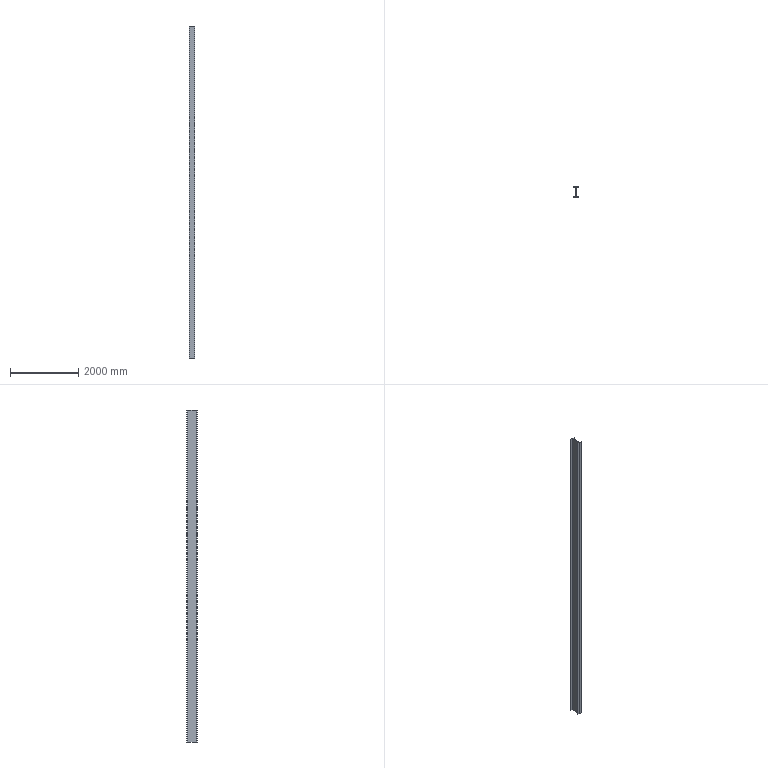Part | SolidWorks | features Extrusion 1 | 1 solid | 18 faces | box 150 x 300 x 9710 mm | volume 45424068 mm3 | plane 14 | cylinder 4 | commonest cylinder face diameters 26 x4
STEP:
#1=CARTESIAN_POINT('',(-75.,9.,0.));
#2=VERTEX_POINT('',#1);
#3=CARTESIAN_POINT('',(-75.,0.,0.));
#4=VERTEX_POINT('',#3);
#5=CARTESIAN_POINT('',(-75.,0.,0.));
#6=DIRECTION('',(0.,-1.,0.));
#7=VECTOR('',#6,1000.);
#8=LINE('',#5,#7);
#9=EDGE_CURVE('',#2,#4,#8,.T.);
#10=ORIENTED_EDGE('',*,*,#9,.T.);
#11=CARTESIAN_POINT('',(-75.,0.,9710.));
#12=VERTEX_POINT('',#11);
#13=CARTESIAN_POINT('',(-75.,0.,9710.));
#14=DIRECTION('',(0.,0.,-1.));
#15=VECTOR('',#14,1000.);
#16=LINE('',#13,#15);
#17=EDGE_CURVE('',#12,#4,#16,.T.);
#18=ORIENTED_EDGE('',*,*,#17,.F.);
#19=CARTESIAN_POINT('',(-75.,9.,9710.));
#20=VERTEX_POINT('',#19);
#21=CARTESIAN_POINT('',(-75.,0.,9710.));
#22=DIRECTION('',(0.,-1.,0.));
#23=VECTOR('',#22,1000.);
#24=LINE('',#21,#23);
#25=EDGE_CURVE('',#20,#12,#24,.T.);
#26=ORIENTED_EDGE('',*,*,#25,.F.);
#27=CARTESIAN_POINT('',(-75.,9.,9710.));
#28=DIRECTION('',(0.,0.,-1.));
#29=VECTOR('',#28,1000.);
#30=LINE('',#27,#29);
#31=EDGE_CURVE('',#20,#2,#30,.T.);
#32=ORIENTED_EDGE('',*,*,#31,.T.);
#33=EDGE_LOOP('',(#10,#18,#26,#32));
#34=FACE_OUTER_BOUND('',#33,.T.);
#35=CARTESIAN_POINT('',(-75.,0.,9710.));
#36=DIRECTION('',(1.,0.,0.));
#37=DIRECTION('',(0.,0.,-1.));
#38=AXIS2_PLACEMENT_3D('',#35,#36,#37);
#39=PLANE('',#38);
#40=ADVANCED_FACE('',(#34),#39,.F.);
#41=CARTESIAN_POINT('',(75.,0.,0.));
#42=VERTEX_POINT('',#41);
#43=CARTESIAN_POINT('',(75.,0.,0.));
#44=DIRECTION('',(1.,0.,0.));
#45=VECTOR('',#44,1000.);
#46=LINE('',#43,#45);
#47=EDGE_CURVE('',#4,#42,#46,.T.);
#48=ORIENTED_EDGE('',*,*,#47,.T.);
#49=CARTESIAN_POINT('',(75.,0.,9710.));
#50=VERTEX_POINT('',#49);
#51=CARTESIAN_POINT('',(75.,0.,9710.));
#52=DIRECTION('',(0.,0.,-1.));
#53=VECTOR('',#52,1000.);
#54=LINE('',#51,#53);
#55=EDGE_CURVE('',#50,#42,#54,.T.);
#56=ORIENTED_EDGE('',*,*,#55,.F.);
#57=CARTESIAN_POINT('',(75.,0.,9710.));
#58=DIRECTION('',(1.,0.,0.));
#59=VECTOR('',#58,1000.);
#60=LINE('',#57,#59);
#61=EDGE_CURVE('',#12,#50,#60,.T.);
#62=ORIENTED_EDGE('',*,*,#61,.F.);
#63=ORIENTED_EDGE('',*,*,#17,.T.);
#64=EDGE_LOOP('',(#48,#56,#62,#63));
#65=FACE_OUTER_BOUND('',#64,.T.);
#66=CARTESIAN_POINT('',(75.,0.,9710.));
#67=DIRECTION('',(0.,1.,0.));
#68=DIRECTION('',(-1.,0.,0.));
#69=AXIS2_PLACEMENT_3D('',#66,#67,#68);
#70=PLANE('',#69);
#71=ADVANCED_FACE('',(#65),#70,.F.);
#72=CARTESIAN_POINT('',(75.,9.,0.));
#73=VERTEX_POINT('',#72);
#74=CARTESIAN_POINT('',(75.,0.,0.));
#75=DIRECTION('',(0.,1.,0.));
#76=VECTOR('',#75,1000.);
#77=LINE('',#74,#76);
#78=EDGE_CURVE('',#42,#73,#77,.T.);
#79=ORIENTED_EDGE('',*,*,#78,.T.);
#80=CARTESIAN_POINT('',(75.,9.,9710.));
#81=VERTEX_POINT('',#80);
#82=CARTESIAN_POINT('',(75.,9.,9710.));
#83=DIRECTION('',(0.,0.,-1.));
#84=VECTOR('',#83,1000.);
#85=LINE('',#82,#84);
#86=EDGE_CURVE('',#81,#73,#85,.T.);
#87=ORIENTED_EDGE('',*,*,#86,.F.);
#88=CARTESIAN_POINT('',(75.,0.,9710.));
#89=DIRECTION('',(0.,1.,0.));
#90=VECTOR('',#89,1000.);
#91=LINE('',#88,#90);
#92=EDGE_CURVE('',#50,#81,#91,.T.);
#93=ORIENTED_EDGE('',*,*,#92,.F.);
#94=ORIENTED_EDGE('',*,*,#55,.T.);
#95=EDGE_LOOP('',(#79,#87,#93,#94));
#96=FACE_OUTER_BOUND('',#95,.T.);
#97=CARTESIAN_POINT('',(75.,0.,9710.));
#98=DIRECTION('',(-1.,0.,0.));
#99=DIRECTION('',(0.,0.,1.));
#100=AXIS2_PLACEMENT_3D('',#97,#98,#99);
#101=PLANE('',#100);
#102=ADVANCED_FACE('',(#96),#101,.F.);
#103=CARTESIAN_POINT('',(16.25,9.,0.));
#104=VERTEX_POINT('',#103);
#105=CARTESIAN_POINT('',(75.,9.,0.));
#106=DIRECTION('',(-1.,0.,0.));
#107=VECTOR('',#106,1000.);
#108=LINE('',#105,#107);
#109=EDGE_CURVE('',#73,#104,#108,.T.);
#110=ORIENTED_EDGE('',*,*,#109,.T.);
#111=CARTESIAN_POINT('',(16.25,9.,9710.));
#112=VERTEX_POINT('',#111);
#113=CARTESIAN_POINT('',(16.25,9.,9710.));
#114=DIRECTION('',(0.,0.,-1.));
#115=VECTOR('',#114,1000.);
#116=LINE('',#113,#115);
#117=EDGE_CURVE('',#112,#104,#116,.T.);
#118=ORIENTED_EDGE('',*,*,#117,.F.);
#119=CARTESIAN_POINT('',(75.,9.,9710.));
#120=DIRECTION('',(-1.,0.,0.));
#121=VECTOR('',#120,1000.);
#122=LINE('',#119,#121);
#123=EDGE_CURVE('',#81,#112,#122,.T.);
#124=ORIENTED_EDGE('',*,*,#123,.F.);
#125=ORIENTED_EDGE('',*,*,#86,.T.);
#126=EDGE_LOOP('',(#110,#118,#124,#125));
#127=FACE_OUTER_BOUND('',#126,.T.);
#128=CARTESIAN_POINT('',(75.,9.,9710.));
#129=DIRECTION('',(0.,-1.,0.));
#130=DIRECTION('',(1.,0.,0.));
#131=AXIS2_PLACEMENT_3D('',#128,#129,#130);
#132=PLANE('',#131);
#133=ADVANCED_FACE('',(#127),#132,.F.);
#134=CARTESIAN_POINT('',(3.25,22.,0.));
#135=VERTEX_POINT('',#134);
#136=CARTESIAN_POINT('',(16.25,22.,0.));
#137=DIRECTION('',(0.,0.,-1.));
#138=DIRECTION('',(-1.,0.,0.));
#139=AXIS2_PLACEMENT_3D('',#136,#137,#138);
#140=CIRCLE('',#139,13.);
#141=EDGE_CURVE('',#104,#135,#140,.T.);
#142=ORIENTED_EDGE('',*,*,#141,.T.);
#143=CARTESIAN_POINT('',(3.25,22.,9710.));
#144=VERTEX_POINT('',#143);
#145=CARTESIAN_POINT('',(3.25,22.,9710.));
#146=DIRECTION('',(0.,0.,-1.));
#147=VECTOR('',#146,1000.);
#148=LINE('',#145,#147);
#149=EDGE_CURVE('',#144,#135,#148,.T.);
#150=ORIENTED_EDGE('',*,*,#149,.F.);
#151=CARTESIAN_POINT('',(16.25,22.,9710.));
#152=DIRECTION('',(0.,0.,-1.));
#153=DIRECTION('',(-1.,0.,0.));
#154=AXIS2_PLACEMENT_3D('',#151,#152,#153);
#155=CIRCLE('',#154,13.);
#156=EDGE_CURVE('',#112,#144,#155,.T.);
#157=ORIENTED_EDGE('',*,*,#156,.F.);
#158=ORIENTED_EDGE('',*,*,#117,.T.);
#159=EDGE_LOOP('',(#142,#150,#157,#158));
#160=FACE_OUTER_BOUND('',#159,.T.);
#161=CARTESIAN_POINT('',(16.25,22.,9710.));
#162=DIRECTION('',(0.,0.,-1.));
#163=DIRECTION('',(-1.,0.,0.));
#164=AXIS2_PLACEMENT_3D('',#161,#162,#163);
#165=CYLINDRICAL_SURFACE('',#164,13.);
#166=ADVANCED_FACE('',(#160),#165,.F.);
#167=CARTESIAN_POINT('',(3.25,278.,0.));
#168=VERTEX_POINT('',#167);
#169=CARTESIAN_POINT('',(3.25,22.,0.));
#170=DIRECTION('',(0.,1.,0.));
#171=VECTOR('',#170,1000.);
#172=LINE('',#169,#171);
#173=EDGE_CURVE('',#135,#168,#172,.T.);
#174=ORIENTED_EDGE('',*,*,#173,.T.);
#175=CARTESIAN_POINT('',(3.25,278.,9710.));
#176=VERTEX_POINT('',#175);
#177=CARTESIAN_POINT('',(3.25,278.,9710.));
#178=DIRECTION('',(0.,0.,-1.));
#179=VECTOR('',#178,1000.);
#180=LINE('',#177,#179);
#181=EDGE_CURVE('',#176,#168,#180,.T.);
#182=ORIENTED_EDGE('',*,*,#181,.F.);
#183=CARTESIAN_POINT('',(3.25,22.,9710.));
#184=DIRECTION('',(0.,1.,0.));
#185=VECTOR('',#184,1000.);
#186=LINE('',#183,#185);
#187=EDGE_CURVE('',#144,#176,#186,.T.);
#188=ORIENTED_EDGE('',*,*,#187,.F.);
#189=ORIENTED_EDGE('',*,*,#149,.T.);
#190=EDGE_LOOP('',(#174,#182,#188,#189));
#191=FACE_OUTER_BOUND('',#190,.T.);
#192=CARTESIAN_POINT('',(3.25,22.,9710.));
#193=DIRECTION('',(-1.,0.,0.));
#194=DIRECTION('',(0.,0.,1.));
#195=AXIS2_PLACEMENT_3D('',#192,#193,#194);
#196=PLANE('',#195);
#197=ADVANCED_FACE('',(#191),#196,.F.);
#198=CARTESIAN_POINT('',(16.25,291.,0.));
#199=VERTEX_POINT('',#198);
#200=CARTESIAN_POINT('',(16.25,278.,0.));
#201=DIRECTION('',(0.,0.,-1.));
#202=DIRECTION('',(-1.,0.,0.));
#203=AXIS2_PLACEMENT_3D('',#200,#201,#202);
#204=CIRCLE('',#203,13.);
#205=EDGE_CURVE('',#168,#199,#204,.T.);
#206=ORIENTED_EDGE('',*,*,#205,.T.);
#207=CARTESIAN_POINT('',(16.25,291.,9710.));
#208=VERTEX_POINT('',#207);
#209=CARTESIAN_POINT('',(16.25,291.,9710.));
#210=DIRECTION('',(0.,0.,-1.));
#211=VECTOR('',#210,1000.);
#212=LINE('',#209,#211);
#213=EDGE_CURVE('',#208,#199,#212,.T.);
#214=ORIENTED_EDGE('',*,*,#213,.F.);
#215=CARTESIAN_POINT('',(16.25,278.,9710.));
#216=DIRECTION('',(0.,0.,-1.));
#217=DIRECTION('',(-1.,0.,0.));
#218=AXIS2_PLACEMENT_3D('',#215,#216,#217);
#219=CIRCLE('',#218,13.);
#220=EDGE_CURVE('',#176,#208,#219,.T.);
#221=ORIENTED_EDGE('',*,*,#220,.F.);
#222=ORIENTED_EDGE('',*,*,#181,.T.);
#223=EDGE_LOOP('',(#206,#214,#221,#222));
#224=FACE_OUTER_BOUND('',#223,.T.);
#225=CARTESIAN_POINT('',(16.25,278.,9710.));
#226=DIRECTION('',(0.,0.,-1.));
#227=DIRECTION('',(-1.,0.,0.));
#228=AXIS2_PLACEMENT_3D('',#225,#226,#227);
#229=CYLINDRICAL_SURFACE('',#228,13.);
#230=ADVANCED_FACE('',(#224),#229,.F.);
#231=CARTESIAN_POINT('',(75.,291.,0.));
#232=VERTEX_POINT('',#231);
#233=CARTESIAN_POINT('',(16.25,291.,0.));
#234=DIRECTION('',(1.,0.,0.));
#235=VECTOR('',#234,1000.);
#236=LINE('',#233,#235);
#237=EDGE_CURVE('',#199,#232,#236,.T.);
#238=ORIENTED_EDGE('',*,*,#237,.T.);
#239=CARTESIAN_POINT('',(75.,291.,9710.));
#240=VERTEX_POINT('',#239);
#241=CARTESIAN_POINT('',(75.,291.,9710.));
#242=DIRECTION('',(0.,0.,-1.));
#243=VECTOR('',#242,1000.);
#244=LINE('',#241,#243);
#245=EDGE_CURVE('',#240,#232,#244,.T.);
#246=ORIENTED_EDGE('',*,*,#245,.F.);
#247=CARTESIAN_POINT('',(16.25,291.,9710.));
#248=DIRECTION('',(1.,0.,0.));
#249=VECTOR('',#248,1000.);
#250=LINE('',#247,#249);
#251=EDGE_CURVE('',#208,#240,#250,.T.);
#252=ORIENTED_EDGE('',*,*,#251,.F.);
#253=ORIENTED_EDGE('',*,*,#213,.T.);
#254=EDGE_LOOP('',(#238,#246,#252,#253));
#255=FACE_OUTER_BOUND('',#254,.T.);
#256=CARTESIAN_POINT('',(16.25,291.,9710.));
#257=DIRECTION('',(0.,1.,0.));
#258=DIRECTION('',(-1.,0.,0.));
#259=AXIS2_PLACEMENT_3D('',#256,#257,#258);
#260=PLANE('',#259);
#261=ADVANCED_FACE('',(#255),#260,.F.);
#262=CARTESIAN_POINT('',(75.,300.,0.));
#263=VERTEX_POINT('',#262);
#264=CARTESIAN_POINT('',(75.,291.,0.));
#265=DIRECTION('',(0.,1.,0.));
#266=VECTOR('',#265,1000.);
#267=LINE('',#264,#266);
#268=EDGE_CURVE('',#232,#263,#267,.T.);
#269=ORIENTED_EDGE('',*,*,#268,.T.);
#270=CARTESIAN_POINT('',(75.,300.,9710.));
#271=VERTEX_POINT('',#270);
#272=CARTESIAN_POINT('',(75.,300.,9710.));
#273=DIRECTION('',(0.,0.,-1.));
#274=VECTOR('',#273,1000.);
#275=LINE('',#272,#274);
#276=EDGE_CURVE('',#271,#263,#275,.T.);
#277=ORIENTED_EDGE('',*,*,#276,.F.);
#278=CARTESIAN_POINT('',(75.,291.,9710.));
#279=DIRECTION('',(0.,1.,0.));
#280=VECTOR('',#279,1000.);
#281=LINE('',#278,#280);
#282=EDGE_CURVE('',#240,#271,#281,.T.);
#283=ORIENTED_EDGE('',*,*,#282,.F.);
#284=ORIENTED_EDGE('',*,*,#245,.T.);
#285=EDGE_LOOP('',(#269,#277,#283,#284));
#286=FACE_OUTER_BOUND('',#285,.T.);
#287=CARTESIAN_POINT('',(75.,291.,9710.));
#288=DIRECTION('',(-1.,0.,0.));
#289=DIRECTION('',(0.,-1.,0.));
#290=AXIS2_PLACEMENT_3D('',#287,#288,#289);
#291=PLANE('',#290);
#292=ADVANCED_FACE('',(#286),#291,.F.);
#293=CARTESIAN_POINT('',(-75.,300.,0.));
#294=VERTEX_POINT('',#293);
#295=CARTESIAN_POINT('',(-75.,300.,0.));
#296=DIRECTION('',(-1.,0.,0.));
#297=VECTOR('',#296,1000.);
#298=LINE('',#295,#297);
#299=EDGE_CURVE('',#263,#294,#298,.T.);
#300=ORIENTED_EDGE('',*,*,#299,.T.);
#301=CARTESIAN_POINT('',(-75.,300.,9710.));
#302=VERTEX_POINT('',#301);
#303=CARTESIAN_POINT('',(-75.,300.,9710.));
#304=DIRECTION('',(0.,0.,-1.));
#305=VECTOR('',#304,1000.);
#306=LINE('',#303,#305);
#307=EDGE_CURVE('',#302,#294,#306,.T.);
#308=ORIENTED_EDGE('',*,*,#307,.F.);
#309=CARTESIAN_POINT('',(-75.,300.,9710.));
#310=DIRECTION('',(-1.,0.,0.));
#311=VECTOR('',#310,1000.);
#312=LINE('',#309,#311);
#313=EDGE_CURVE('',#271,#302,#312,.T.);
#314=ORIENTED_EDGE('',*,*,#313,.F.);
#315=ORIENTED_EDGE('',*,*,#276,.T.);
#316=EDGE_LOOP('',(#300,#308,#314,#315));
#317=FACE_OUTER_BOUND('',#316,.T.);
#318=CARTESIAN_POINT('',(-75.,300.,9710.));
#319=DIRECTION('',(0.,-1.,0.));
#320=DIRECTION('',(0.,0.,-1.));
#321=AXIS2_PLACEMENT_3D('',#318,#319,#320);
#322=PLANE('',#321);
#323=ADVANCED_FACE('',(#317),#322,.F.);
#324=CARTESIAN_POINT('',(-75.,291.,0.));
#325=VERTEX_POINT('',#324);
#326=CARTESIAN_POINT('',(-75.,291.,0.));
#327=DIRECTION('',(0.,-1.,0.));
#328=VECTOR('',#327,1000.);
#329=LINE('',#326,#328);
#330=EDGE_CURVE('',#294,#325,#329,.T.);
#331=ORIENTED_EDGE('',*,*,#330,.T.);
#332=CARTESIAN_POINT('',(-75.,291.,9710.));
#333=VERTEX_POINT('',#332);
#334=CARTESIAN_POINT('',(-75.,291.,9710.));
#335=DIRECTION('',(0.,0.,-1.));
#336=VECTOR('',#335,1000.);
#337=LINE('',#334,#336);
#338=EDGE_CURVE('',#333,#325,#337,.T.);
#339=ORIENTED_EDGE('',*,*,#338,.F.);
#340=CARTESIAN_POINT('',(-75.,291.,9710.));
#341=DIRECTION('',(0.,-1.,0.));
#342=VECTOR('',#341,1000.);
#343=LINE('',#340,#342);
#344=EDGE_CURVE('',#302,#333,#343,.T.);
#345=ORIENTED_EDGE('',*,*,#344,.F.);
#346=ORIENTED_EDGE('',*,*,#307,.T.);
#347=EDGE_LOOP('',(#331,#339,#345,#346));
#348=FACE_OUTER_BOUND('',#347,.T.);
#349=CARTESIAN_POINT('',(-75.,291.,9710.));
#350=DIRECTION('',(1.,0.,0.));
#351=DIRECTION('',(0.,1.,0.));
#352=AXIS2_PLACEMENT_3D('',#349,#350,#351);
#353=PLANE('',#352);
#354=ADVANCED_FACE('',(#348),#353,.F.);
#355=CARTESIAN_POINT('',(-16.25,291.,0.));
#356=VERTEX_POINT('',#355);
#357=CARTESIAN_POINT('',(-16.25,291.,0.));
#358=DIRECTION('',(1.,0.,0.));
#359=VECTOR('',#358,1000.);
#360=LINE('',#357,#359);
#361=EDGE_CURVE('',#325,#356,#360,.T.);
#362=ORIENTED_EDGE('',*,*,#361,.T.);
#363=CARTESIAN_POINT('',(-16.25,291.,9710.));
#364=VERTEX_POINT('',#363);
#365=CARTESIAN_POINT('',(-16.25,291.,9710.));
#366=DIRECTION('',(0.,0.,-1.));
#367=VECTOR('',#366,1000.);
#368=LINE('',#365,#367);
#369=EDGE_CURVE('',#364,#356,#368,.T.);
#370=ORIENTED_EDGE('',*,*,#369,.F.);
#371=CARTESIAN_POINT('',(-16.25,291.,9710.));
#372=DIRECTION('',(1.,0.,0.));
#373=VECTOR('',#372,1000.);
#374=LINE('',#371,#373);
#375=EDGE_CURVE('',#333,#364,#374,.T.);
#376=ORIENTED_EDGE('',*,*,#375,.F.);
#377=ORIENTED_EDGE('',*,*,#338,.T.);
#378=EDGE_LOOP('',(#362,#370,#376,#377));
#379=FACE_OUTER_BOUND('',#378,.T.);
#380=CARTESIAN_POINT('',(-16.25,291.,9710.));
#381=DIRECTION('',(0.,1.,0.));
#382=DIRECTION('',(-1.,0.,0.));
#383=AXIS2_PLACEMENT_3D('',#380,#381,#382);
#384=PLANE('',#383);
#385=ADVANCED_FACE('',(#379),#384,.F.);
#386=CARTESIAN_POINT('',(-3.25,278.,0.));
#387=VERTEX_POINT('',#386);
#388=CARTESIAN_POINT('',(-16.25,278.,0.));
#389=DIRECTION('',(0.,0.,-1.));
#390=DIRECTION('',(1.,0.,0.));
#391=AXIS2_PLACEMENT_3D('',#388,#389,#390);
#392=CIRCLE('',#391,13.);
#393=EDGE_CURVE('',#356,#387,#392,.T.);
#394=ORIENTED_EDGE('',*,*,#393,.T.);
#395=CARTESIAN_POINT('',(-3.25,278.,9710.));
#396=VERTEX_POINT('',#395);
#397=CARTESIAN_POINT('',(-3.25,278.,9710.));
#398=DIRECTION('',(0.,0.,-1.));
#399=VECTOR('',#398,1000.);
#400=LINE('',#397,#399);
#401=EDGE_CURVE('',#396,#387,#400,.T.);
#402=ORIENTED_EDGE('',*,*,#401,.F.);
#403=CARTESIAN_POINT('',(-16.25,278.,9710.));
#404=DIRECTION('',(0.,0.,-1.));
#405=DIRECTION('',(1.,0.,0.));
#406=AXIS2_PLACEMENT_3D('',#403,#404,#405);
#407=CIRCLE('',#406,13.);
#408=EDGE_CURVE('',#364,#396,#407,.T.);
#409=ORIENTED_EDGE('',*,*,#408,.F.);
#410=ORIENTED_EDGE('',*,*,#369,.T.);
#411=EDGE_LOOP('',(#394,#402,#409,#410));
#412=FACE_OUTER_BOUND('',#411,.T.);
#413=CARTESIAN_POINT('',(-16.25,278.,9710.));
#414=DIRECTION('',(0.,0.,-1.));
#415=DIRECTION('',(-1.,0.,0.));
#416=AXIS2_PLACEMENT_3D('',#413,#414,#415);
#417=CYLINDRICAL_SURFACE('',#416,13.);
#418=ADVANCED_FACE('',(#412),#417,.F.);
#419=CARTESIAN_POINT('',(-3.25,22.,0.));
#420=VERTEX_POINT('',#419);
#421=CARTESIAN_POINT('',(-3.25,22.,0.));
#422=DIRECTION('',(0.,-1.,0.));
#423=VECTOR('',#422,1000.);
#424=LINE('',#421,#423);
#425=EDGE_CURVE('',#387,#420,#424,.T.);
#426=ORIENTED_EDGE('',*,*,#425,.T.);
#427=CARTESIAN_POINT('',(-3.25,22.,9710.));
#428=VERTEX_POINT('',#427);
#429=CARTESIAN_POINT('',(-3.25,22.,9710.));
#430=DIRECTION('',(0.,0.,-1.));
#431=VECTOR('',#430,1000.);
#432=LINE('',#429,#431);
#433=EDGE_CURVE('',#428,#420,#432,.T.);
#434=ORIENTED_EDGE('',*,*,#433,.F.);
#435=CARTESIAN_POINT('',(-3.25,22.,9710.));
#436=DIRECTION('',(0.,-1.,0.));
#437=VECTOR('',#436,1000.);
#438=LINE('',#435,#437);
#439=EDGE_CURVE('',#396,#428,#438,.T.);
#440=ORIENTED_EDGE('',*,*,#439,.F.);
#441=ORIENTED_EDGE('',*,*,#401,.T.);
#442=EDGE_LOOP('',(#426,#434,#440,#441));
#443=FACE_OUTER_BOUND('',#442,.T.);
#444=CARTESIAN_POINT('',(-3.25,22.,9710.));
#445=DIRECTION('',(1.,0.,0.));
#446=DIRECTION('',(0.,0.,-1.));
#447=AXIS2_PLACEMENT_3D('',#444,#445,#446);
#448=PLANE('',#447);
#449=ADVANCED_FACE('',(#443),#448,.F.);
#450=CARTESIAN_POINT('',(-16.25,9.,0.));
#451=VERTEX_POINT('',#450);
#452=CARTESIAN_POINT('',(-16.25,22.,0.));
#453=DIRECTION('',(0.,0.,-1.));
#454=DIRECTION('',(-1.,0.,0.));
#455=AXIS2_PLACEMENT_3D('',#452,#453,#454);
#456=CIRCLE('',#455,13.);
#457=EDGE_CURVE('',#420,#451,#456,.T.);
#458=ORIENTED_EDGE('',*,*,#457,.T.);
#459=CARTESIAN_POINT('',(-16.25,9.,9710.));
#460=VERTEX_POINT('',#459);
#461=CARTESIAN_POINT('',(-16.25,9.,9710.));
#462=DIRECTION('',(0.,0.,-1.));
#463=VECTOR('',#462,1000.);
#464=LINE('',#461,#463);
#465=EDGE_CURVE('',#460,#451,#464,.T.);
#466=ORIENTED_EDGE('',*,*,#465,.F.);
#467=CARTESIAN_POINT('',(-16.25,22.,9710.));
#468=DIRECTION('',(0.,0.,-1.));
#469=DIRECTION('',(-1.,0.,0.));
#470=AXIS2_PLACEMENT_3D('',#467,#468,#469);
#471=CIRCLE('',#470,13.);
#472=EDGE_CURVE('',#428,#460,#471,.T.);
#473=ORIENTED_EDGE('',*,*,#472,.F.);
#474=ORIENTED_EDGE('',*,*,#433,.T.);
#475=EDGE_LOOP('',(#458,#466,#473,#474));
#476=FACE_OUTER_BOUND('',#475,.T.);
#477=CARTESIAN_POINT('',(-16.25,22.,9710.));
#478=DIRECTION('',(0.,0.,-1.));
#479=DIRECTION('',(-1.,0.,0.));
#480=AXIS2_PLACEMENT_3D('',#477,#478,#479);
#481=CYLINDRICAL_SURFACE('',#480,13.);
#482=ADVANCED_FACE('',(#476),#481,.F.);
#483=CARTESIAN_POINT('',(-75.,9.,0.));
#484=DIRECTION('',(-1.,0.,0.));
#485=VECTOR('',#484,1000.);
#486=LINE('',#483,#485);
#487=EDGE_CURVE('',#451,#2,#486,.T.);
#488=ORIENTED_EDGE('',*,*,#487,.T.);
#489=ORIENTED_EDGE('',*,*,#31,.F.);
#490=CARTESIAN_POINT('',(-75.,9.,9710.));
#491=DIRECTION('',(-1.,0.,0.));
#492=VECTOR('',#491,1000.);
#493=LINE('',#490,#492);
#494=EDGE_CURVE('',#460,#20,#493,.T.);
#495=ORIENTED_EDGE('',*,*,#494,.F.);
#496=ORIENTED_EDGE('',*,*,#465,.T.);
#497=EDGE_LOOP('',(#488,#489,#495,#496));
#498=FACE_OUTER_BOUND('',#497,.T.);
#499=CARTESIAN_POINT('',(-75.,9.,9710.));
#500=DIRECTION('',(0.,-1.,0.));
#501=DIRECTION('',(1.,0.,0.));
#502=AXIS2_PLACEMENT_3D('',#499,#500,#501);
#503=PLANE('',#502);
#504=ADVANCED_FACE('',(#498),#503,.F.);
#505=ORIENTED_EDGE('',*,*,#25,.T.);
#506=ORIENTED_EDGE('',*,*,#61,.T.);
#507=ORIENTED_EDGE('',*,*,#92,.T.);
#508=ORIENTED_EDGE('',*,*,#123,.T.);
#509=ORIENTED_EDGE('',*,*,#156,.T.);
#510=ORIENTED_EDGE('',*,*,#187,.T.);
#511=ORIENTED_EDGE('',*,*,#220,.T.);
#512=ORIENTED_EDGE('',*,*,#251,.T.);
#513=ORIENTED_EDGE('',*,*,#282,.T.);
#514=ORIENTED_EDGE('',*,*,#313,.T.);
#515=ORIENTED_EDGE('',*,*,#344,.T.);
#516=ORIENTED_EDGE('',*,*,#375,.T.);
#517=ORIENTED_EDGE('',*,*,#408,.T.);
#518=ORIENTED_EDGE('',*,*,#439,.T.);
#519=ORIENTED_EDGE('',*,*,#472,.T.);
#520=ORIENTED_EDGE('',*,*,#494,.T.);
#521=EDGE_LOOP('',(#505,#506,#507,#508,#509,#510,#511,#512,#513,#514,#515,#516,#517,#518,#519,#520));
#522=FACE_OUTER_BOUND('',#521,.T.);
#523=CARTESIAN_POINT('',(-16.25,22.,9710.));
#524=DIRECTION('',(0.,0.,-1.));
#525=DIRECTION('',(-1.,0.,0.));
#526=AXIS2_PLACEMENT_3D('',#523,#524,#525);
#527=PLANE('',#526);
#528=ADVANCED_FACE('',(#522),#527,.F.);
#529=ORIENTED_EDGE('',*,*,#9,.F.);
#530=ORIENTED_EDGE('',*,*,#487,.F.);
#531=ORIENTED_EDGE('',*,*,#457,.F.);
#532=ORIENTED_EDGE('',*,*,#425,.F.);
#533=ORIENTED_EDGE('',*,*,#393,.F.);
#534=ORIENTED_EDGE('',*,*,#361,.F.);
#535=ORIENTED_EDGE('',*,*,#330,.F.);
#536=ORIENTED_EDGE('',*,*,#299,.F.);
#537=ORIENTED_EDGE('',*,*,#268,.F.);
#538=ORIENTED_EDGE('',*,*,#237,.F.);
#539=ORIENTED_EDGE('',*,*,#205,.F.);
#540=ORIENTED_EDGE('',*,*,#173,.F.);
#541=ORIENTED_EDGE('',*,*,#141,.F.);
#542=ORIENTED_EDGE('',*,*,#109,.F.);
#543=ORIENTED_EDGE('',*,*,#78,.F.);
#544=ORIENTED_EDGE('',*,*,#47,.F.);
#545=EDGE_LOOP('',(#529,#530,#531,#532,#533,#534,#535,#536,#537,#538,#539,#540,#541,#542,#543,#544));
#546=FACE_OUTER_BOUND('',#545,.T.);
#547=CARTESIAN_POINT('',(-16.25,22.,0.));
#548=DIRECTION('',(0.,0.,-1.));
#549=DIRECTION('',(-1.,0.,0.));
#550=AXIS2_PLACEMENT_3D('',#547,#548,#549);
#551=PLANE('',#550);
#552=ADVANCED_FACE('',(#546),#551,.T.);
#553=CLOSED_SHELL('',(#40,#71,#102,#133,#166,#197,#230,#261,#292,#323,#354,#385,#418,#449,#482,#504,#528,#552));
#554=MANIFOLD_SOLID_BREP('',#553);
#555=CARTESIAN_POINT('',(0.,0.,0.));
#556=DIRECTION('',(0.,0.,1.));
#557=DIRECTION('',(1.,0.,0.));
#558=AXIS2_PLACEMENT_3D('',#555,#556,#557);
#559=(LENGTH_UNIT()NAMED_UNIT(*)SI_UNIT(.MILLI.,.METRE.));
#560=UNCERTAINTY_MEASURE_WITH_UNIT(LENGTH_MEASURE(0.00001),#559,'','');
#561=(NAMED_UNIT(*)PLANE_ANGLE_UNIT()SI_UNIT($,.RADIAN.));
#562=(NAMED_UNIT(*)SI_UNIT($,.STERADIAN.)SOLID_ANGLE_UNIT());
#563=(GEOMETRIC_REPRESENTATION_CONTEXT(3)GLOBAL_UNCERTAINTY_ASSIGNED_CONTEXT((#560))GLOBAL_UNIT_ASSIGNED_CONTEXT((#559,#561,#562))REPRESENTATION_CONTEXT('',''));
#564=ADVANCED_BREP_SHAPE_REPRESENTATION('',(#554,#558),#563);